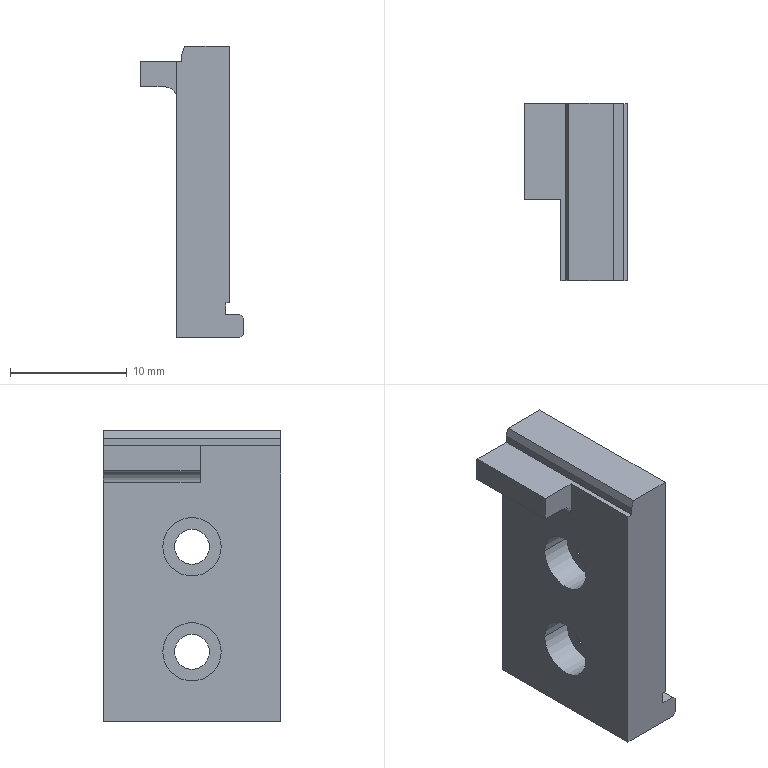Part | NX | 1 solid | 29 faces | box 8.8 x 15.2 x 25 mm | volume 1656 mm3 | plane 20 | cylinder 9 | commonest cylinder face diameters 3 x4 5 x4 2 x1
STEP:
#1=CARTESIAN_POINT('',(1.77,0.,1.43));
#2=VERTEX_POINT('',#1);
#3=CARTESIAN_POINT('',(1.77,0.,0.78));
#4=VERTEX_POINT('',#3);
#5=CARTESIAN_POINT('',(1.77,0.,0.));
#6=DIRECTION('',(0.,0.,-1.));
#7=VECTOR('',#6,1000.);
#8=LINE('',#5,#7);
#9=EDGE_CURVE('',#2,#4,#8,.T.);
#10=ORIENTED_EDGE('',*,*,#9,.T.);
#11=CARTESIAN_POINT('',(1.35,0.,0.78));
#12=VERTEX_POINT('',#11);
#13=CARTESIAN_POINT('',(0.,0.,0.78));
#14=DIRECTION('',(-1.,0.,0.));
#15=VECTOR('',#14,1000.);
#16=LINE('',#13,#15);
#17=EDGE_CURVE('',#4,#12,#16,.T.);
#18=ORIENTED_EDGE('',*,*,#17,.T.);
#19=CARTESIAN_POINT('',(1.35,0.,-22.87));
#20=VERTEX_POINT('',#19);
#21=CARTESIAN_POINT('',(1.35,0.,0.));
#22=DIRECTION('',(0.,0.,1.));
#23=VECTOR('',#22,1000.);
#24=LINE('',#21,#23);
#25=EDGE_CURVE('',#20,#12,#24,.T.);
#26=ORIENTED_EDGE('',*,*,#25,.F.);
#27=CARTESIAN_POINT('',(6.75,0.,-22.87));
#28=VERTEX_POINT('',#27);
#29=CARTESIAN_POINT('',(0.,0.,-22.87));
#30=DIRECTION('',(1.,0.,0.));
#31=VECTOR('',#30,1000.);
#32=LINE('',#29,#31);
#33=EDGE_CURVE('',#20,#28,#32,.T.);
#34=ORIENTED_EDGE('',*,*,#33,.T.);
#35=CARTESIAN_POINT('',(7.05,0.,-22.57));
#36=VERTEX_POINT('',#35);
#37=CARTESIAN_POINT('',(29.62,0.,0.));
#38=DIRECTION('',(0.7071,0.,0.7071));
#39=VECTOR('',#38,1000.);
#40=LINE('',#37,#39);
#41=EDGE_CURVE('',#28,#36,#40,.T.);
#42=ORIENTED_EDGE('',*,*,#41,.T.);
#43=CARTESIAN_POINT('',(7.05,0.,-21.17));
#44=VERTEX_POINT('',#43);
#45=CARTESIAN_POINT('',(7.05,0.,0.));
#46=DIRECTION('',(0.,0.,1.));
#47=VECTOR('',#46,1000.);
#48=LINE('',#45,#47);
#49=EDGE_CURVE('',#36,#44,#48,.T.);
#50=ORIENTED_EDGE('',*,*,#49,.T.);
#51=CARTESIAN_POINT('',(6.75,0.,-20.87));
#52=VERTEX_POINT('',#51);
#53=CARTESIAN_POINT('',(-14.12,0.,0.));
#54=DIRECTION('',(0.7071,0.,-0.7071));
#55=VECTOR('',#54,1000.);
#56=LINE('',#53,#55);
#57=EDGE_CURVE('',#52,#44,#56,.T.);
#58=ORIENTED_EDGE('',*,*,#57,.F.);
#59=CARTESIAN_POINT('',(5.55,0.,-20.87));
#60=VERTEX_POINT('',#59);
#61=CARTESIAN_POINT('',(0.,0.,-20.87));
#62=DIRECTION('',(-1.,0.,0.));
#63=VECTOR('',#62,1000.);
#64=LINE('',#61,#63);
#65=EDGE_CURVE('',#52,#60,#64,.T.);
#66=ORIENTED_EDGE('',*,*,#65,.T.);
#67=CARTESIAN_POINT('',(5.55,0.,-19.87));
#68=VERTEX_POINT('',#67);
#69=CARTESIAN_POINT('',(5.55,0.,0.));
#70=DIRECTION('',(0.,0.,1.));
#71=VECTOR('',#70,1000.);
#72=LINE('',#69,#71);
#73=EDGE_CURVE('',#60,#68,#72,.T.);
#74=ORIENTED_EDGE('',*,*,#73,.T.);
#75=CARTESIAN_POINT('',(5.85,0.,-19.87));
#76=VERTEX_POINT('',#75);
#77=CARTESIAN_POINT('',(0.,0.,-19.87));
#78=DIRECTION('',(1.,0.,0.));
#79=VECTOR('',#78,1000.);
#80=LINE('',#77,#79);
#81=EDGE_CURVE('',#68,#76,#80,.T.);
#82=ORIENTED_EDGE('',*,*,#81,.T.);
#83=CARTESIAN_POINT('',(5.85,0.,2.13));
#84=VERTEX_POINT('',#83);
#85=CARTESIAN_POINT('',(5.85,0.,0.));
#86=DIRECTION('',(0.,0.,1.));
#87=VECTOR('',#86,1000.);
#88=LINE('',#85,#87);
#89=EDGE_CURVE('',#76,#84,#88,.T.);
#90=ORIENTED_EDGE('',*,*,#89,.T.);
#91=CARTESIAN_POINT('',(2.025,0.,2.13));
#92=VERTEX_POINT('',#91);
#93=CARTESIAN_POINT('',(0.,0.,2.13));
#94=DIRECTION('',(1.,0.,0.));
#95=VECTOR('',#94,1000.);
#96=LINE('',#93,#95);
#97=EDGE_CURVE('',#92,#84,#96,.T.);
#98=ORIENTED_EDGE('',*,*,#97,.F.);
#99=CARTESIAN_POINT('',(1.25,0.,0.));
#100=DIRECTION('',(-0.342,0.,-0.9397));
#101=VECTOR('',#100,1000.);
#102=LINE('',#99,#101);
#103=EDGE_CURVE('',#92,#2,#102,.T.);
#104=ORIENTED_EDGE('',*,*,#103,.T.);
#105=EDGE_LOOP('',(#10,#18,#26,#34,#42,#50,#58,#66,#74,#82,#90,#98,#104));
#106=FACE_BOUND('',#105,.T.);
#107=CARTESIAN_POINT('',(0.,0.,0.));
#108=DIRECTION('',(0.,-1.,0.));
#109=DIRECTION('',(0.,0.,-1.));
#110=AXIS2_PLACEMENT_3D('',#107,#108,#109);
#111=PLANE('',#110);
#112=ADVANCED_FACE('',(#106),#111,.T.);
#113=CARTESIAN_POINT('',(1.77,15.2,0.78));
#114=VERTEX_POINT('',#113);
#115=CARTESIAN_POINT('',(1.77,15.2,1.43));
#116=VERTEX_POINT('',#115);
#117=CARTESIAN_POINT('',(1.77,15.2,0.));
#118=DIRECTION('',(0.,0.,1.));
#119=VECTOR('',#118,1000.);
#120=LINE('',#117,#119);
#121=EDGE_CURVE('',#114,#116,#120,.T.);
#122=ORIENTED_EDGE('',*,*,#121,.F.);
#123=CARTESIAN_POINT('',(1.77,0.,0.78));
#124=DIRECTION('',(0.,1.,0.));
#125=VECTOR('',#124,1000.);
#126=LINE('',#123,#125);
#127=EDGE_CURVE('',#4,#114,#126,.T.);
#128=ORIENTED_EDGE('',*,*,#127,.F.);
#129=ORIENTED_EDGE('',*,*,#9,.F.);
#130=CARTESIAN_POINT('',(1.77,0.,1.43));
#131=DIRECTION('',(0.,-1.,0.));
#132=VECTOR('',#131,1000.);
#133=LINE('',#130,#132);
#134=EDGE_CURVE('',#116,#2,#133,.T.);
#135=ORIENTED_EDGE('',*,*,#134,.F.);
#136=EDGE_LOOP('',(#122,#128,#129,#135));
#137=FACE_BOUND('',#136,.T.);
#138=CARTESIAN_POINT('',(1.77,0.,0.93));
#139=DIRECTION('',(1.,0.,0.));
#140=DIRECTION('',(0.,1.,0.));
#141=AXIS2_PLACEMENT_3D('',#138,#139,#140);
#142=PLANE('',#141);
#143=ADVANCED_FACE('',(#137),#142,.F.);
#144=CARTESIAN_POINT('',(-1.75,15.2,0.78));
#145=VERTEX_POINT('',#144);
#146=CARTESIAN_POINT('',(-1.75,15.2,-1.37));
#147=VERTEX_POINT('',#146);
#148=CARTESIAN_POINT('',(-1.75,15.2,0.));
#149=DIRECTION('',(0.,0.,-1.));
#150=VECTOR('',#149,1000.);
#151=LINE('',#148,#150);
#152=EDGE_CURVE('',#145,#147,#151,.T.);
#153=ORIENTED_EDGE('',*,*,#152,.F.);
#154=CARTESIAN_POINT('',(0.,15.2,0.78));
#155=DIRECTION('',(1.,0.,0.));
#156=VECTOR('',#155,1000.);
#157=LINE('',#154,#156);
#158=EDGE_CURVE('',#145,#114,#157,.T.);
#159=ORIENTED_EDGE('',*,*,#158,.T.);
#160=ORIENTED_EDGE('',*,*,#121,.T.);
#161=CARTESIAN_POINT('',(2.025,15.2,2.13));
#162=VERTEX_POINT('',#161);
#163=CARTESIAN_POINT('',(1.25,15.2,0.));
#164=DIRECTION('',(0.342,0.,0.9397));
#165=VECTOR('',#164,1000.);
#166=LINE('',#163,#165);
#167=EDGE_CURVE('',#116,#162,#166,.T.);
#168=ORIENTED_EDGE('',*,*,#167,.T.);
#169=CARTESIAN_POINT('',(5.85,15.2,2.13));
#170=VERTEX_POINT('',#169);
#171=CARTESIAN_POINT('',(0.,15.2,2.13));
#172=DIRECTION('',(-1.,0.,0.));
#173=VECTOR('',#172,1000.);
#174=LINE('',#171,#173);
#175=EDGE_CURVE('',#170,#162,#174,.T.);
#176=ORIENTED_EDGE('',*,*,#175,.F.);
#177=CARTESIAN_POINT('',(5.85,15.2,-19.87));
#178=VERTEX_POINT('',#177);
#179=CARTESIAN_POINT('',(5.85,15.2,0.));
#180=DIRECTION('',(0.,0.,-1.));
#181=VECTOR('',#180,1000.);
#182=LINE('',#179,#181);
#183=EDGE_CURVE('',#170,#178,#182,.T.);
#184=ORIENTED_EDGE('',*,*,#183,.T.);
#185=CARTESIAN_POINT('',(5.55,15.2,-19.87));
#186=VERTEX_POINT('',#185);
#187=CARTESIAN_POINT('',(0.,15.2,-19.87));
#188=DIRECTION('',(-1.,0.,0.));
#189=VECTOR('',#188,1000.);
#190=LINE('',#187,#189);
#191=EDGE_CURVE('',#178,#186,#190,.T.);
#192=ORIENTED_EDGE('',*,*,#191,.T.);
#193=CARTESIAN_POINT('',(5.55,15.2,-20.87));
#194=VERTEX_POINT('',#193);
#195=CARTESIAN_POINT('',(5.55,15.2,0.));
#196=DIRECTION('',(0.,0.,-1.));
#197=VECTOR('',#196,1000.);
#198=LINE('',#195,#197);
#199=EDGE_CURVE('',#186,#194,#198,.T.);
#200=ORIENTED_EDGE('',*,*,#199,.T.);
#201=CARTESIAN_POINT('',(6.75,15.2,-20.87));
#202=VERTEX_POINT('',#201);
#203=CARTESIAN_POINT('',(0.,15.2,-20.87));
#204=DIRECTION('',(-1.,0.,0.));
#205=VECTOR('',#204,1000.);
#206=LINE('',#203,#205);
#207=EDGE_CURVE('',#202,#194,#206,.T.);
#208=ORIENTED_EDGE('',*,*,#207,.F.);
#209=CARTESIAN_POINT('',(7.05,15.2,-21.17));
#210=VERTEX_POINT('',#209);
#211=CARTESIAN_POINT('',(-14.12,15.2,0.));
#212=DIRECTION('',(-0.7071,0.,0.7071));
#213=VECTOR('',#212,1000.);
#214=LINE('',#211,#213);
#215=EDGE_CURVE('',#210,#202,#214,.T.);
#216=ORIENTED_EDGE('',*,*,#215,.F.);
#217=CARTESIAN_POINT('',(7.05,15.2,-22.57));
#218=VERTEX_POINT('',#217);
#219=CARTESIAN_POINT('',(7.05,15.2,0.));
#220=DIRECTION('',(0.,0.,1.));
#221=VECTOR('',#220,1000.);
#222=LINE('',#219,#221);
#223=EDGE_CURVE('',#218,#210,#222,.T.);
#224=ORIENTED_EDGE('',*,*,#223,.F.);
#225=CARTESIAN_POINT('',(6.75,15.2,-22.87));
#226=VERTEX_POINT('',#225);
#227=CARTESIAN_POINT('',(29.62,15.2,0.));
#228=DIRECTION('',(-0.7071,0.,-0.7071));
#229=VECTOR('',#228,1000.);
#230=LINE('',#227,#229);
#231=EDGE_CURVE('',#218,#226,#230,.T.);
#232=ORIENTED_EDGE('',*,*,#231,.T.);
#233=CARTESIAN_POINT('',(1.35,15.2,-22.87));
#234=VERTEX_POINT('',#233);
#235=CARTESIAN_POINT('',(0.,15.2,-22.87));
#236=DIRECTION('',(1.,0.,0.));
#237=VECTOR('',#236,1000.);
#238=LINE('',#235,#237);
#239=EDGE_CURVE('',#234,#226,#238,.T.);
#240=ORIENTED_EDGE('',*,*,#239,.F.);
#241=CARTESIAN_POINT('',(1.35,15.2,-2.37));
#242=VERTEX_POINT('',#241);
#243=CARTESIAN_POINT('',(1.35,15.2,0.));
#244=DIRECTION('',(0.,0.,-1.));
#245=VECTOR('',#244,1000.);
#246=LINE('',#243,#245);
#247=EDGE_CURVE('',#242,#234,#246,.T.);
#248=ORIENTED_EDGE('',*,*,#247,.F.);
#249=CARTESIAN_POINT('',(0.35,15.2,-1.37));
#250=VERTEX_POINT('',#249);
#251=CARTESIAN_POINT('',(0.35,15.2,-2.37));
#252=DIRECTION('',(0.,-1.,0.));
#253=DIRECTION('',(1.,0.,0.));
#254=AXIS2_PLACEMENT_3D('',#251,#252,#253);
#255=CIRCLE('',#254,1.);
#256=EDGE_CURVE('',#242,#250,#255,.T.);
#257=ORIENTED_EDGE('',*,*,#256,.T.);
#258=CARTESIAN_POINT('',(0.,15.2,-1.37));
#259=DIRECTION('',(1.,0.,0.));
#260=VECTOR('',#259,1000.);
#261=LINE('',#258,#260);
#262=EDGE_CURVE('',#147,#250,#261,.T.);
#263=ORIENTED_EDGE('',*,*,#262,.F.);
#264=EDGE_LOOP('',(#153,#159,#160,#168,#176,#184,#192,#200,#208,#216,#224,#232,#240,#248,#257,#263));
#265=FACE_BOUND('',#264,.T.);
#266=CARTESIAN_POINT('',(1.35,15.2,0.));
#267=DIRECTION('',(0.,1.,0.));
#268=DIRECTION('',(1.,0.,0.));
#269=AXIS2_PLACEMENT_3D('',#266,#267,#268);
#270=PLANE('',#269);
#271=ADVANCED_FACE('',(#265),#270,.T.);
#272=CARTESIAN_POINT('',(4.05,10.1,-16.87));
#273=VERTEX_POINT('',#272);
#274=CARTESIAN_POINT('',(4.05,5.1,-16.87));
#275=VERTEX_POINT('',#274);
#276=CARTESIAN_POINT('',(4.05,7.6,-16.87));
#277=DIRECTION('',(1.,0.,0.));
#278=DIRECTION('',(0.,1.,0.));
#279=AXIS2_PLACEMENT_3D('',#276,#277,#278);
#280=CIRCLE('',#279,2.5);
#281=EDGE_CURVE('',#273,#275,#280,.T.);
#282=ORIENTED_EDGE('',*,*,#281,.F.);
#283=CARTESIAN_POINT('',(4.05,7.6,-16.87));
#284=DIRECTION('',(1.,0.,0.));
#285=DIRECTION('',(0.,1.,0.));
#286=AXIS2_PLACEMENT_3D('',#283,#284,#285);
#287=CIRCLE('',#286,2.5);
#288=EDGE_CURVE('',#275,#273,#287,.T.);
#289=ORIENTED_EDGE('',*,*,#288,.F.);
#290=EDGE_LOOP('',(#282,#289));
#291=FACE_BOUND('',#290,.T.);
#292=CARTESIAN_POINT('',(4.05,6.1,-16.87));
#293=VERTEX_POINT('',#292);
#294=CARTESIAN_POINT('',(4.05,9.1,-16.87));
#295=VERTEX_POINT('',#294);
#296=CARTESIAN_POINT('',(4.05,7.6,-16.87));
#297=DIRECTION('',(-1.,0.,0.));
#298=DIRECTION('',(0.,1.,0.));
#299=AXIS2_PLACEMENT_3D('',#296,#297,#298);
#300=CIRCLE('',#299,1.5);
#301=EDGE_CURVE('',#293,#295,#300,.T.);
#302=ORIENTED_EDGE('',*,*,#301,.F.);
#303=CARTESIAN_POINT('',(4.05,7.6,-16.87));
#304=DIRECTION('',(-1.,0.,0.));
#305=DIRECTION('',(0.,1.,0.));
#306=AXIS2_PLACEMENT_3D('',#303,#304,#305);
#307=CIRCLE('',#306,1.5);
#308=EDGE_CURVE('',#295,#293,#307,.T.);
#309=ORIENTED_EDGE('',*,*,#308,.F.);
#310=EDGE_LOOP('',(#302,#309));
#311=FACE_BOUND('',#310,.T.);
#312=CARTESIAN_POINT('',(4.05,7.6,-16.87));
#313=DIRECTION('',(-1.,0.,0.));
#314=DIRECTION('',(0.,0.,1.));
#315=AXIS2_PLACEMENT_3D('',#312,#313,#314);
#316=PLANE('',#315);
#317=ADVANCED_FACE('',(#291,#311),#316,.T.);
#318=CARTESIAN_POINT('',(2.025,0.,2.13));
#319=DIRECTION('',(0.,-1.,0.));
#320=VECTOR('',#319,1000.);
#321=LINE('',#318,#320);
#322=EDGE_CURVE('',#162,#92,#321,.T.);
#323=ORIENTED_EDGE('',*,*,#322,.T.);
#324=ORIENTED_EDGE('',*,*,#97,.T.);
#325=CARTESIAN_POINT('',(5.85,0.,2.13));
#326=DIRECTION('',(0.,1.,0.));
#327=VECTOR('',#326,1000.);
#328=LINE('',#325,#327);
#329=EDGE_CURVE('',#84,#170,#328,.T.);
#330=ORIENTED_EDGE('',*,*,#329,.T.);
#331=ORIENTED_EDGE('',*,*,#175,.T.);
#332=EDGE_LOOP('',(#323,#324,#330,#331));
#333=FACE_BOUND('',#332,.T.);
#334=CARTESIAN_POINT('',(0.,0.,2.13));
#335=DIRECTION('',(0.,0.,1.));
#336=DIRECTION('',(1.,0.,0.));
#337=AXIS2_PLACEMENT_3D('',#334,#335,#336);
#338=PLANE('',#337);
#339=ADVANCED_FACE('',(#333),#338,.T.);
#340=ORIENTED_EDGE('',*,*,#322,.F.);
#341=ORIENTED_EDGE('',*,*,#167,.F.);
#342=ORIENTED_EDGE('',*,*,#134,.T.);
#343=ORIENTED_EDGE('',*,*,#103,.F.);
#344=EDGE_LOOP('',(#340,#341,#342,#343));
#345=FACE_BOUND('',#344,.T.);
#346=CARTESIAN_POINT('',(2.025,15.2,2.13));
#347=DIRECTION('',(0.9397,0.,-0.342));
#348=DIRECTION('',(0.,-1.,0.));
#349=AXIS2_PLACEMENT_3D('',#346,#347,#348);
#350=PLANE('',#349);
#351=ADVANCED_FACE('',(#345),#350,.F.);
#352=ORIENTED_EDGE('',*,*,#81,.F.);
#353=CARTESIAN_POINT('',(5.55,0.,-19.87));
#354=DIRECTION('',(0.,-1.,0.));
#355=VECTOR('',#354,1000.);
#356=LINE('',#353,#355);
#357=EDGE_CURVE('',#186,#68,#356,.T.);
#358=ORIENTED_EDGE('',*,*,#357,.F.);
#359=ORIENTED_EDGE('',*,*,#191,.F.);
#360=CARTESIAN_POINT('',(5.85,0.,-19.87));
#361=DIRECTION('',(0.,1.,0.));
#362=VECTOR('',#361,1000.);
#363=LINE('',#360,#362);
#364=EDGE_CURVE('',#76,#178,#363,.T.);
#365=ORIENTED_EDGE('',*,*,#364,.F.);
#366=EDGE_LOOP('',(#352,#358,#359,#365));
#367=FACE_BOUND('',#366,.T.);
#368=CARTESIAN_POINT('',(4.85,0.,-19.87));
#369=DIRECTION('',(0.,0.,1.));
#370=DIRECTION('',(1.,0.,0.));
#371=AXIS2_PLACEMENT_3D('',#368,#369,#370);
#372=PLANE('',#371);
#373=ADVANCED_FACE('',(#367),#372,.F.);
#374=ORIENTED_EDGE('',*,*,#73,.F.);
#375=CARTESIAN_POINT('',(5.55,0.,-20.87));
#376=DIRECTION('',(0.,-1.,0.));
#377=VECTOR('',#376,1000.);
#378=LINE('',#375,#377);
#379=EDGE_CURVE('',#194,#60,#378,.T.);
#380=ORIENTED_EDGE('',*,*,#379,.F.);
#381=ORIENTED_EDGE('',*,*,#199,.F.);
#382=ORIENTED_EDGE('',*,*,#357,.T.);
#383=EDGE_LOOP('',(#374,#380,#381,#382));
#384=FACE_BOUND('',#383,.T.);
#385=CARTESIAN_POINT('',(5.55,0.,-19.87));
#386=DIRECTION('',(-1.,0.,0.));
#387=DIRECTION('',(0.,0.,1.));
#388=AXIS2_PLACEMENT_3D('',#385,#386,#387);
#389=PLANE('',#388);
#390=ADVANCED_FACE('',(#384),#389,.F.);
#391=CARTESIAN_POINT('',(6.75,0.,-20.87));
#392=DIRECTION('',(0.,1.,0.));
#393=VECTOR('',#392,1000.);
#394=LINE('',#391,#393);
#395=EDGE_CURVE('',#52,#202,#394,.T.);
#396=ORIENTED_EDGE('',*,*,#395,.T.);
#397=ORIENTED_EDGE('',*,*,#207,.T.);
#398=ORIENTED_EDGE('',*,*,#379,.T.);
#399=ORIENTED_EDGE('',*,*,#65,.F.);
#400=EDGE_LOOP('',(#396,#397,#398,#399));
#401=FACE_BOUND('',#400,.T.);
#402=CARTESIAN_POINT('',(4.85,0.,-20.87));
#403=DIRECTION('',(0.,0.,-1.));
#404=DIRECTION('',(0.,-1.,0.));
#405=AXIS2_PLACEMENT_3D('',#402,#403,#404);
#406=PLANE('',#405);
#407=ADVANCED_FACE('',(#401),#406,.F.);
#408=CARTESIAN_POINT('',(7.05,0.,-22.57));
#409=DIRECTION('',(0.,-1.,0.));
#410=VECTOR('',#409,1000.);
#411=LINE('',#408,#410);
#412=EDGE_CURVE('',#218,#36,#411,.T.);
#413=ORIENTED_EDGE('',*,*,#412,.F.);
#414=ORIENTED_EDGE('',*,*,#223,.T.);
#415=CARTESIAN_POINT('',(7.05,0.,-21.17));
#416=DIRECTION('',(0.,-1.,0.));
#417=VECTOR('',#416,1000.);
#418=LINE('',#415,#417);
#419=EDGE_CURVE('',#210,#44,#418,.T.);
#420=ORIENTED_EDGE('',*,*,#419,.T.);
#421=ORIENTED_EDGE('',*,*,#49,.F.);
#422=EDGE_LOOP('',(#413,#414,#420,#421));
#423=FACE_BOUND('',#422,.T.);
#424=CARTESIAN_POINT('',(7.05,0.,-20.87));
#425=DIRECTION('',(-1.,0.,0.));
#426=DIRECTION('',(0.,0.,1.));
#427=AXIS2_PLACEMENT_3D('',#424,#425,#426);
#428=PLANE('',#427);
#429=ADVANCED_FACE('',(#423),#428,.F.);
#430=ORIENTED_EDGE('',*,*,#33,.F.);
#431=CARTESIAN_POINT('',(1.35,0.,-22.87));
#432=DIRECTION('',(0.,1.,0.));
#433=VECTOR('',#432,1000.);
#434=LINE('',#431,#433);
#435=EDGE_CURVE('',#20,#234,#434,.T.);
#436=ORIENTED_EDGE('',*,*,#435,.T.);
#437=ORIENTED_EDGE('',*,*,#239,.T.);
#438=CARTESIAN_POINT('',(6.75,0.,-22.87));
#439=DIRECTION('',(0.,1.,0.));
#440=VECTOR('',#439,1000.);
#441=LINE('',#438,#440);
#442=EDGE_CURVE('',#28,#226,#441,.T.);
#443=ORIENTED_EDGE('',*,*,#442,.F.);
#444=EDGE_LOOP('',(#430,#436,#437,#443));
#445=FACE_BOUND('',#444,.T.);
#446=CARTESIAN_POINT('',(6.05,0.,-22.87));
#447=DIRECTION('',(0.,0.,1.));
#448=DIRECTION('',(1.,0.,0.));
#449=AXIS2_PLACEMENT_3D('',#446,#447,#448);
#450=PLANE('',#449);
#451=ADVANCED_FACE('',(#445),#450,.F.);
#452=ORIENTED_EDGE('',*,*,#89,.F.);
#453=ORIENTED_EDGE('',*,*,#364,.T.);
#454=ORIENTED_EDGE('',*,*,#183,.F.);
#455=ORIENTED_EDGE('',*,*,#329,.F.);
#456=EDGE_LOOP('',(#452,#453,#454,#455));
#457=FACE_BOUND('',#456,.T.);
#458=CARTESIAN_POINT('',(5.85,6.1,-16.87));
#459=VERTEX_POINT('',#458);
#460=CARTESIAN_POINT('',(5.85,9.1,-16.87));
#461=VERTEX_POINT('',#460);
#462=CARTESIAN_POINT('',(5.85,7.6,-16.87));
#463=DIRECTION('',(-1.,0.,0.));
#464=DIRECTION('',(0.,1.,0.));
#465=AXIS2_PLACEMENT_3D('',#462,#463,#464);
#466=CIRCLE('',#465,1.5);
#467=EDGE_CURVE('',#459,#461,#466,.T.);
#468=ORIENTED_EDGE('',*,*,#467,.T.);
#469=CARTESIAN_POINT('',(5.85,7.6,-16.87));
#470=DIRECTION('',(-1.,0.,0.));
#471=DIRECTION('',(0.,1.,0.));
#472=AXIS2_PLACEMENT_3D('',#469,#470,#471);
#473=CIRCLE('',#472,1.5);
#474=EDGE_CURVE('',#461,#459,#473,.T.);
#475=ORIENTED_EDGE('',*,*,#474,.T.);
#476=EDGE_LOOP('',(#468,#475));
#477=FACE_BOUND('',#476,.T.);
#478=CARTESIAN_POINT('',(5.85,6.1,-7.87));
#479=VERTEX_POINT('',#478);
#480=CARTESIAN_POINT('',(5.85,9.1,-7.87));
#481=VERTEX_POINT('',#480);
#482=CARTESIAN_POINT('',(5.85,7.6,-7.87));
#483=DIRECTION('',(-1.,0.,0.));
#484=DIRECTION('',(0.,1.,0.));
#485=AXIS2_PLACEMENT_3D('',#482,#483,#484);
#486=CIRCLE('',#485,1.5);
#487=EDGE_CURVE('',#479,#481,#486,.T.);
#488=ORIENTED_EDGE('',*,*,#487,.T.);
#489=CARTESIAN_POINT('',(5.85,7.6,-7.87));
#490=DIRECTION('',(-1.,0.,0.));
#491=DIRECTION('',(0.,1.,0.));
#492=AXIS2_PLACEMENT_3D('',#489,#490,#491);
#493=CIRCLE('',#492,1.5);
#494=EDGE_CURVE('',#481,#479,#493,.T.);
#495=ORIENTED_EDGE('',*,*,#494,.T.);
#496=EDGE_LOOP('',(#488,#495));
#497=FACE_BOUND('',#496,.T.);
#498=CARTESIAN_POINT('',(5.85,0.,1.13));
#499=DIRECTION('',(-1.,0.,0.));
#500=DIRECTION('',(0.,0.,1.));
#501=AXIS2_PLACEMENT_3D('',#498,#499,#500);
#502=PLANE('',#501);
#503=ADVANCED_FACE('',(#457,#477,#497),#502,.F.);
#504=CARTESIAN_POINT('',(1.35,6.9,-2.37));
#505=VERTEX_POINT('',#504);
#506=CARTESIAN_POINT('',(0.35,6.9,-1.37));
#507=VERTEX_POINT('',#506);
#508=CARTESIAN_POINT('',(0.35,6.9,-2.37));
#509=DIRECTION('',(0.,-1.,0.));
#510=DIRECTION('',(1.,0.,0.));
#511=AXIS2_PLACEMENT_3D('',#508,#509,#510);
#512=CIRCLE('',#511,1.);
#513=EDGE_CURVE('',#505,#507,#512,.T.);
#514=ORIENTED_EDGE('',*,*,#513,.T.);
#515=CARTESIAN_POINT('',(0.35,15.2,-1.37));
#516=DIRECTION('',(0.,-1.,0.));
#517=VECTOR('',#516,1000.);
#518=LINE('',#515,#517);
#519=EDGE_CURVE('',#250,#507,#518,.T.);
#520=ORIENTED_EDGE('',*,*,#519,.F.);
#521=ORIENTED_EDGE('',*,*,#256,.F.);
#522=CARTESIAN_POINT('',(1.35,15.285,-2.37));
#523=DIRECTION('',(0.,-1.,0.));
#524=VECTOR('',#523,1000.);
#525=LINE('',#522,#524);
#526=EDGE_CURVE('',#242,#505,#525,.T.);
#527=ORIENTED_EDGE('',*,*,#526,.T.);
#528=EDGE_LOOP('',(#514,#520,#521,#527));
#529=FACE_BOUND('',#528,.T.);
#530=CARTESIAN_POINT('',(0.35,15.285,-2.37));
#531=DIRECTION('',(0.,-1.,0.));
#532=DIRECTION('',(1.,0.,0.));
#533=AXIS2_PLACEMENT_3D('',#530,#531,#532);
#534=CYLINDRICAL_SURFACE('',#533,1.);
#535=ADVANCED_FACE('',(#529),#534,.F.);
#536=CARTESIAN_POINT('',(-1.75,6.9,-1.37));
#537=VERTEX_POINT('',#536);
#538=CARTESIAN_POINT('',(0.,6.9,-1.37));
#539=DIRECTION('',(1.,0.,0.));
#540=VECTOR('',#539,1000.);
#541=LINE('',#538,#540);
#542=EDGE_CURVE('',#537,#507,#541,.T.);
#543=ORIENTED_EDGE('',*,*,#542,.T.);
#544=ORIENTED_EDGE('',*,*,#513,.F.);
#545=CARTESIAN_POINT('',(1.35,6.9,0.78));
#546=VERTEX_POINT('',#545);
#547=CARTESIAN_POINT('',(1.35,6.9,0.));
#548=DIRECTION('',(0.,0.,1.));
#549=VECTOR('',#548,1000.);
#550=LINE('',#547,#549);
#551=EDGE_CURVE('',#505,#546,#550,.T.);
#552=ORIENTED_EDGE('',*,*,#551,.T.);
#553=CARTESIAN_POINT('',(-1.75,6.9,0.78));
#554=VERTEX_POINT('',#553);
#555=CARTESIAN_POINT('',(0.,6.9,0.78));
#556=DIRECTION('',(1.,0.,0.));
#557=VECTOR('',#556,1000.);
#558=LINE('',#555,#557);
#559=EDGE_CURVE('',#554,#546,#558,.T.);
#560=ORIENTED_EDGE('',*,*,#559,.F.);
#561=CARTESIAN_POINT('',(-1.75,6.9,0.));
#562=DIRECTION('',(0.,0.,-1.));
#563=VECTOR('',#562,1000.);
#564=LINE('',#561,#563);
#565=EDGE_CURVE('',#554,#537,#564,.T.);
#566=ORIENTED_EDGE('',*,*,#565,.T.);
#567=EDGE_LOOP('',(#543,#544,#552,#560,#566));
#568=FACE_BOUND('',#567,.T.);
#569=CARTESIAN_POINT('',(1.77,6.9,0.83));
#570=DIRECTION('',(0.,-1.,0.));
#571=DIRECTION('',(0.,0.,-1.));
#572=AXIS2_PLACEMENT_3D('',#569,#570,#571);
#573=PLANE('',#572);
#574=ADVANCED_FACE('',(#568),#573,.T.);
#575=CARTESIAN_POINT('',(-1.75,0.,-1.37));
#576=DIRECTION('',(0.,1.,0.));
#577=VECTOR('',#576,1000.);
#578=LINE('',#575,#577);
#579=EDGE_CURVE('',#537,#147,#578,.T.);
#580=ORIENTED_EDGE('',*,*,#579,.F.);
#581=ORIENTED_EDGE('',*,*,#565,.F.);
#582=CARTESIAN_POINT('',(-1.75,0.,0.78));
#583=DIRECTION('',(0.,-1.,0.));
#584=VECTOR('',#583,1000.);
#585=LINE('',#582,#584);
#586=EDGE_CURVE('',#145,#554,#585,.T.);
#587=ORIENTED_EDGE('',*,*,#586,.F.);
#588=ORIENTED_EDGE('',*,*,#152,.T.);
#589=EDGE_LOOP('',(#580,#581,#587,#588));
#590=FACE_BOUND('',#589,.T.);
#591=CARTESIAN_POINT('',(-1.75,0.,-52.77));
#592=DIRECTION('',(-1.,0.,0.));
#593=DIRECTION('',(0.,0.,1.));
#594=AXIS2_PLACEMENT_3D('',#591,#592,#593);
#595=PLANE('',#594);
#596=ADVANCED_FACE('',(#590),#595,.T.);
#597=CARTESIAN_POINT('',(1.35,10.1,-7.87));
#598=VERTEX_POINT('',#597);
#599=CARTESIAN_POINT('',(1.35,5.1,-7.87));
#600=VERTEX_POINT('',#599);
#601=CARTESIAN_POINT('',(1.35,7.6,-7.87));
#602=DIRECTION('',(-1.,0.,0.));
#603=DIRECTION('',(0.,1.,0.));
#604=AXIS2_PLACEMENT_3D('',#601,#602,#603);
#605=CIRCLE('',#604,2.5);
#606=EDGE_CURVE('',#598,#600,#605,.T.);
#607=ORIENTED_EDGE('',*,*,#606,.T.);
#608=CARTESIAN_POINT('',(4.05,5.1,-7.87));
#609=VERTEX_POINT('',#608);
#610=CARTESIAN_POINT('',(7.072,5.1,-7.87));
#611=DIRECTION('',(-1.,0.,0.));
#612=VECTOR('',#611,1000.);
#613=LINE('',#610,#612);
#614=EDGE_CURVE('',#609,#600,#613,.T.);
#615=ORIENTED_EDGE('',*,*,#614,.F.);
#616=CARTESIAN_POINT('',(4.05,10.1,-7.87));
#617=VERTEX_POINT('',#616);
#618=CARTESIAN_POINT('',(4.05,7.6,-7.87));
#619=DIRECTION('',(1.,0.,0.));
#620=DIRECTION('',(0.,1.,0.));
#621=AXIS2_PLACEMENT_3D('',#618,#619,#620);
#622=CIRCLE('',#621,2.5);
#623=EDGE_CURVE('',#609,#617,#622,.T.);
#624=ORIENTED_EDGE('',*,*,#623,.T.);
#625=CARTESIAN_POINT('',(7.072,10.1,-7.87));
#626=DIRECTION('',(-1.,0.,0.));
#627=VECTOR('',#626,1000.);
#628=LINE('',#625,#627);
#629=EDGE_CURVE('',#617,#598,#628,.T.);
#630=ORIENTED_EDGE('',*,*,#629,.T.);
#631=EDGE_LOOP('',(#607,#615,#624,#630));
#632=FACE_BOUND('',#631,.T.);
#633=CARTESIAN_POINT('',(7.072,7.6,-7.87));
#634=DIRECTION('',(-1.,0.,0.));
#635=DIRECTION('',(0.,1.,0.));
#636=AXIS2_PLACEMENT_3D('',#633,#634,#635);
#637=CYLINDRICAL_SURFACE('',#636,2.5);
#638=ADVANCED_FACE('',(#632),#637,.F.);
#639=ORIENTED_EDGE('',*,*,#579,.T.);
#640=ORIENTED_EDGE('',*,*,#262,.T.);
#641=ORIENTED_EDGE('',*,*,#519,.T.);
#642=ORIENTED_EDGE('',*,*,#542,.F.);
#643=EDGE_LOOP('',(#639,#640,#641,#642));
#644=FACE_BOUND('',#643,.T.);
#645=CARTESIAN_POINT('',(1.35,15.2,-1.37));
#646=DIRECTION('',(0.,0.,-1.));
#647=DIRECTION('',(0.,-1.,0.));
#648=AXIS2_PLACEMENT_3D('',#645,#646,#647);
#649=PLANE('',#648);
#650=ADVANCED_FACE('',(#644),#649,.T.);
#651=ORIENTED_EDGE('',*,*,#158,.F.);
#652=ORIENTED_EDGE('',*,*,#586,.T.);
#653=ORIENTED_EDGE('',*,*,#559,.T.);
#654=CARTESIAN_POINT('',(1.35,0.,0.78));
#655=DIRECTION('',(0.,-1.,0.));
#656=VECTOR('',#655,1000.);
#657=LINE('',#654,#656);
#658=EDGE_CURVE('',#546,#12,#657,.T.);
#659=ORIENTED_EDGE('',*,*,#658,.T.);
#660=ORIENTED_EDGE('',*,*,#17,.F.);
#661=ORIENTED_EDGE('',*,*,#127,.T.);
#662=EDGE_LOOP('',(#651,#652,#653,#659,#660,#661));
#663=FACE_BOUND('',#662,.T.);
#664=CARTESIAN_POINT('',(-1.45,0.,0.78));
#665=DIRECTION('',(0.,0.,-1.));
#666=DIRECTION('',(0.,-1.,0.));
#667=AXIS2_PLACEMENT_3D('',#664,#665,#666);
#668=PLANE('',#667);
#669=ADVANCED_FACE('',(#663),#668,.F.);
#670=CARTESIAN_POINT('',(4.05,6.1,-7.87));
#671=VERTEX_POINT('',#670);
#672=CARTESIAN_POINT('',(4.05,9.1,-7.87));
#673=VERTEX_POINT('',#672);
#674=CARTESIAN_POINT('',(4.05,7.6,-7.87));
#675=DIRECTION('',(-1.,0.,0.));
#676=DIRECTION('',(0.,1.,0.));
#677=AXIS2_PLACEMENT_3D('',#674,#675,#676);
#678=CIRCLE('',#677,1.5);
#679=EDGE_CURVE('',#671,#673,#678,.T.);
#680=ORIENTED_EDGE('',*,*,#679,.T.);
#681=CARTESIAN_POINT('',(7.072,9.1,-7.87));
#682=DIRECTION('',(-1.,0.,0.));
#683=VECTOR('',#682,1000.);
#684=LINE('',#681,#683);
#685=EDGE_CURVE('',#481,#673,#684,.T.);
#686=ORIENTED_EDGE('',*,*,#685,.F.);
#687=ORIENTED_EDGE('',*,*,#487,.F.);
#688=CARTESIAN_POINT('',(7.072,6.1,-7.87));
#689=DIRECTION('',(-1.,0.,0.));
#690=VECTOR('',#689,1000.);
#691=LINE('',#688,#690);
#692=EDGE_CURVE('',#479,#671,#691,.T.);
#693=ORIENTED_EDGE('',*,*,#692,.T.);
#694=EDGE_LOOP('',(#680,#686,#687,#693));
#695=FACE_BOUND('',#694,.T.);
#696=CARTESIAN_POINT('',(7.072,7.6,-7.87));
#697=DIRECTION('',(-1.,0.,0.));
#698=DIRECTION('',(0.,1.,0.));
#699=AXIS2_PLACEMENT_3D('',#696,#697,#698);
#700=CYLINDRICAL_SURFACE('',#699,1.5);
#701=ADVANCED_FACE('',(#695),#700,.F.);
#702=ORIENTED_EDGE('',*,*,#301,.T.);
#703=CARTESIAN_POINT('',(7.072,9.1,-16.87));
#704=DIRECTION('',(-1.,0.,0.));
#705=VECTOR('',#704,1000.);
#706=LINE('',#703,#705);
#707=EDGE_CURVE('',#461,#295,#706,.T.);
#708=ORIENTED_EDGE('',*,*,#707,.F.);
#709=ORIENTED_EDGE('',*,*,#467,.F.);
#710=CARTESIAN_POINT('',(7.072,6.1,-16.87));
#711=DIRECTION('',(-1.,0.,0.));
#712=VECTOR('',#711,1000.);
#713=LINE('',#710,#712);
#714=EDGE_CURVE('',#459,#293,#713,.T.);
#715=ORIENTED_EDGE('',*,*,#714,.T.);
#716=EDGE_LOOP('',(#702,#708,#709,#715));
#717=FACE_BOUND('',#716,.T.);
#718=CARTESIAN_POINT('',(7.072,7.6,-16.87));
#719=DIRECTION('',(-1.,0.,0.));
#720=DIRECTION('',(0.,1.,0.));
#721=AXIS2_PLACEMENT_3D('',#718,#719,#720);
#722=CYLINDRICAL_SURFACE('',#721,1.5);
#723=ADVANCED_FACE('',(#717),#722,.F.);
#724=CARTESIAN_POINT('',(1.35,5.1,-16.87));
#725=VERTEX_POINT('',#724);
#726=CARTESIAN_POINT('',(1.35,10.1,-16.87));
#727=VERTEX_POINT('',#726);
#728=CARTESIAN_POINT('',(1.35,7.6,-16.87));
#729=DIRECTION('',(-1.,0.,0.));
#730=DIRECTION('',(0.,1.,0.));
#731=AXIS2_PLACEMENT_3D('',#728,#729,#730);
#732=CIRCLE('',#731,2.5);
#733=EDGE_CURVE('',#725,#727,#732,.T.);
#734=ORIENTED_EDGE('',*,*,#733,.T.);
#735=CARTESIAN_POINT('',(7.072,10.1,-16.87));
#736=DIRECTION('',(-1.,0.,0.));
#737=VECTOR('',#736,1000.);
#738=LINE('',#735,#737);
#739=EDGE_CURVE('',#273,#727,#738,.T.);
#740=ORIENTED_EDGE('',*,*,#739,.F.);
#741=ORIENTED_EDGE('',*,*,#281,.T.);
#742=CARTESIAN_POINT('',(7.072,5.1,-16.87));
#743=DIRECTION('',(-1.,0.,0.));
#744=VECTOR('',#743,1000.);
#745=LINE('',#742,#744);
#746=EDGE_CURVE('',#275,#725,#745,.T.);
#747=ORIENTED_EDGE('',*,*,#746,.T.);
#748=EDGE_LOOP('',(#734,#740,#741,#747));
#749=FACE_BOUND('',#748,.T.);
#750=CARTESIAN_POINT('',(7.072,7.6,-16.87));
#751=DIRECTION('',(-1.,0.,0.));
#752=DIRECTION('',(0.,1.,0.));
#753=AXIS2_PLACEMENT_3D('',#750,#751,#752);
#754=CYLINDRICAL_SURFACE('',#753,2.5);
#755=ADVANCED_FACE('',(#749),#754,.F.);
#756=ORIENTED_EDGE('',*,*,#435,.F.);
#757=ORIENTED_EDGE('',*,*,#25,.T.);
#758=ORIENTED_EDGE('',*,*,#658,.F.);
#759=ORIENTED_EDGE('',*,*,#551,.F.);
#760=ORIENTED_EDGE('',*,*,#526,.F.);
#761=ORIENTED_EDGE('',*,*,#247,.T.);
#762=EDGE_LOOP('',(#756,#757,#758,#759,#760,#761));
#763=FACE_BOUND('',#762,.T.);
#764=ORIENTED_EDGE('',*,*,#733,.F.);
#765=CARTESIAN_POINT('',(1.35,7.6,-16.87));
#766=DIRECTION('',(-1.,0.,0.));
#767=DIRECTION('',(0.,1.,0.));
#768=AXIS2_PLACEMENT_3D('',#765,#766,#767);
#769=CIRCLE('',#768,2.5);
#770=EDGE_CURVE('',#727,#725,#769,.T.);
#771=ORIENTED_EDGE('',*,*,#770,.F.);
#772=EDGE_LOOP('',(#764,#771));
#773=FACE_BOUND('',#772,.T.);
#774=ORIENTED_EDGE('',*,*,#606,.F.);
#775=CARTESIAN_POINT('',(1.35,7.6,-7.87));
#776=DIRECTION('',(-1.,0.,0.));
#777=DIRECTION('',(0.,1.,0.));
#778=AXIS2_PLACEMENT_3D('',#775,#776,#777);
#779=CIRCLE('',#778,2.5);
#780=EDGE_CURVE('',#600,#598,#779,.T.);
#781=ORIENTED_EDGE('',*,*,#780,.F.);
#782=EDGE_LOOP('',(#774,#781));
#783=FACE_BOUND('',#782,.T.);
#784=CARTESIAN_POINT('',(1.35,0.,1.13));
#785=DIRECTION('',(-1.,0.,0.));
#786=DIRECTION('',(0.,0.,1.));
#787=AXIS2_PLACEMENT_3D('',#784,#785,#786);
#788=PLANE('',#787);
#789=ADVANCED_FACE('',(#763,#773,#783),#788,.T.);
#790=ORIENTED_EDGE('',*,*,#623,.F.);
#791=CARTESIAN_POINT('',(4.05,7.6,-7.87));
#792=DIRECTION('',(1.,0.,0.));
#793=DIRECTION('',(0.,1.,0.));
#794=AXIS2_PLACEMENT_3D('',#791,#792,#793);
#795=CIRCLE('',#794,2.5);
#796=EDGE_CURVE('',#617,#609,#795,.T.);
#797=ORIENTED_EDGE('',*,*,#796,.F.);
#798=EDGE_LOOP('',(#790,#797));
#799=FACE_BOUND('',#798,.T.);
#800=ORIENTED_EDGE('',*,*,#679,.F.);
#801=CARTESIAN_POINT('',(4.05,7.6,-7.87));
#802=DIRECTION('',(-1.,0.,0.));
#803=DIRECTION('',(0.,1.,0.));
#804=AXIS2_PLACEMENT_3D('',#801,#802,#803);
#805=CIRCLE('',#804,1.5);
#806=EDGE_CURVE('',#673,#671,#805,.T.);
#807=ORIENTED_EDGE('',*,*,#806,.F.);
#808=EDGE_LOOP('',(#800,#807));
#809=FACE_BOUND('',#808,.T.);
#810=CARTESIAN_POINT('',(4.05,7.6,-7.87));
#811=DIRECTION('',(-1.,0.,0.));
#812=DIRECTION('',(0.,0.,1.));
#813=AXIS2_PLACEMENT_3D('',#810,#811,#812);
#814=PLANE('',#813);
#815=ADVANCED_FACE('',(#799,#809),#814,.T.);
#816=ORIENTED_EDGE('',*,*,#412,.T.);
#817=ORIENTED_EDGE('',*,*,#41,.F.);
#818=ORIENTED_EDGE('',*,*,#442,.T.);
#819=ORIENTED_EDGE('',*,*,#231,.F.);
#820=EDGE_LOOP('',(#816,#817,#818,#819));
#821=FACE_BOUND('',#820,.T.);
#822=CARTESIAN_POINT('',(6.9,7.6,-22.72));
#823=DIRECTION('',(-0.7071,0.,0.7071));
#824=DIRECTION('',(0.,1.,0.));
#825=AXIS2_PLACEMENT_3D('',#822,#823,#824);
#826=PLANE('',#825);
#827=ADVANCED_FACE('',(#821),#826,.F.);
#828=ORIENTED_EDGE('',*,*,#395,.F.);
#829=ORIENTED_EDGE('',*,*,#57,.T.);
#830=ORIENTED_EDGE('',*,*,#419,.F.);
#831=ORIENTED_EDGE('',*,*,#215,.T.);
#832=EDGE_LOOP('',(#828,#829,#830,#831));
#833=FACE_BOUND('',#832,.T.);
#834=CARTESIAN_POINT('',(6.9,7.6,-21.02));
#835=DIRECTION('',(0.7071,0.,0.7071));
#836=DIRECTION('',(0.,-1.,0.));
#837=AXIS2_PLACEMENT_3D('',#834,#835,#836);
#838=PLANE('',#837);
#839=ADVANCED_FACE('',(#833),#838,.T.);
#840=ORIENTED_EDGE('',*,*,#739,.T.);
#841=ORIENTED_EDGE('',*,*,#770,.T.);
#842=ORIENTED_EDGE('',*,*,#746,.F.);
#843=ORIENTED_EDGE('',*,*,#288,.T.);
#844=EDGE_LOOP('',(#840,#841,#842,#843));
#845=FACE_BOUND('',#844,.T.);
#846=CARTESIAN_POINT('',(7.072,7.6,-16.87));
#847=DIRECTION('',(-1.,0.,0.));
#848=DIRECTION('',(0.,1.,0.));
#849=AXIS2_PLACEMENT_3D('',#846,#847,#848);
#850=CYLINDRICAL_SURFACE('',#849,2.5);
#851=ADVANCED_FACE('',(#845),#850,.F.);
#852=ORIENTED_EDGE('',*,*,#629,.F.);
#853=ORIENTED_EDGE('',*,*,#796,.T.);
#854=ORIENTED_EDGE('',*,*,#614,.T.);
#855=ORIENTED_EDGE('',*,*,#780,.T.);
#856=EDGE_LOOP('',(#852,#853,#854,#855));
#857=FACE_BOUND('',#856,.T.);
#858=CARTESIAN_POINT('',(7.072,7.6,-7.87));
#859=DIRECTION('',(-1.,0.,0.));
#860=DIRECTION('',(0.,1.,0.));
#861=AXIS2_PLACEMENT_3D('',#858,#859,#860);
#862=CYLINDRICAL_SURFACE('',#861,2.5);
#863=ADVANCED_FACE('',(#857),#862,.F.);
#864=ORIENTED_EDGE('',*,*,#685,.T.);
#865=ORIENTED_EDGE('',*,*,#806,.T.);
#866=ORIENTED_EDGE('',*,*,#692,.F.);
#867=ORIENTED_EDGE('',*,*,#494,.F.);
#868=EDGE_LOOP('',(#864,#865,#866,#867));
#869=FACE_BOUND('',#868,.T.);
#870=CARTESIAN_POINT('',(7.072,7.6,-7.87));
#871=DIRECTION('',(-1.,0.,0.));
#872=DIRECTION('',(0.,1.,0.));
#873=AXIS2_PLACEMENT_3D('',#870,#871,#872);
#874=CYLINDRICAL_SURFACE('',#873,1.5);
#875=ADVANCED_FACE('',(#869),#874,.F.);
#876=ORIENTED_EDGE('',*,*,#707,.T.);
#877=ORIENTED_EDGE('',*,*,#308,.T.);
#878=ORIENTED_EDGE('',*,*,#714,.F.);
#879=ORIENTED_EDGE('',*,*,#474,.F.);
#880=EDGE_LOOP('',(#876,#877,#878,#879));
#881=FACE_BOUND('',#880,.T.);
#882=CARTESIAN_POINT('',(7.072,7.6,-16.87));
#883=DIRECTION('',(-1.,0.,0.));
#884=DIRECTION('',(0.,1.,0.));
#885=AXIS2_PLACEMENT_3D('',#882,#883,#884);
#886=CYLINDRICAL_SURFACE('',#885,1.5);
#887=ADVANCED_FACE('',(#881),#886,.F.);
#888=CLOSED_SHELL('',(#112,#143,#271,#317,#339,#351,#373,#390,#407,#429,#451,#503,#535,#574,#596,#638,#650,#669,#701,#723,#755,#789,#815,#827,#839,#851,#863,#875,#887));
#889=MANIFOLD_SOLID_BREP('',#888);
#890=(LENGTH_UNIT()NAMED_UNIT(*)SI_UNIT(.MILLI.,.METRE.));
#891=UNCERTAINTY_MEASURE_WITH_UNIT(LENGTH_MEASURE(0.00001),#890,'','');
#892=(NAMED_UNIT(*)PLANE_ANGLE_UNIT()SI_UNIT($,.RADIAN.));
#893=(NAMED_UNIT(*)SI_UNIT($,.STERADIAN.)SOLID_ANGLE_UNIT());
#894=(GEOMETRIC_REPRESENTATION_CONTEXT(3)GLOBAL_UNCERTAINTY_ASSIGNED_CONTEXT((#891))GLOBAL_UNIT_ASSIGNED_CONTEXT((#890,#892,#893))REPRESENTATION_CONTEXT('',''));
#895=ADVANCED_BREP_SHAPE_REPRESENTATION('',(#889),#894);